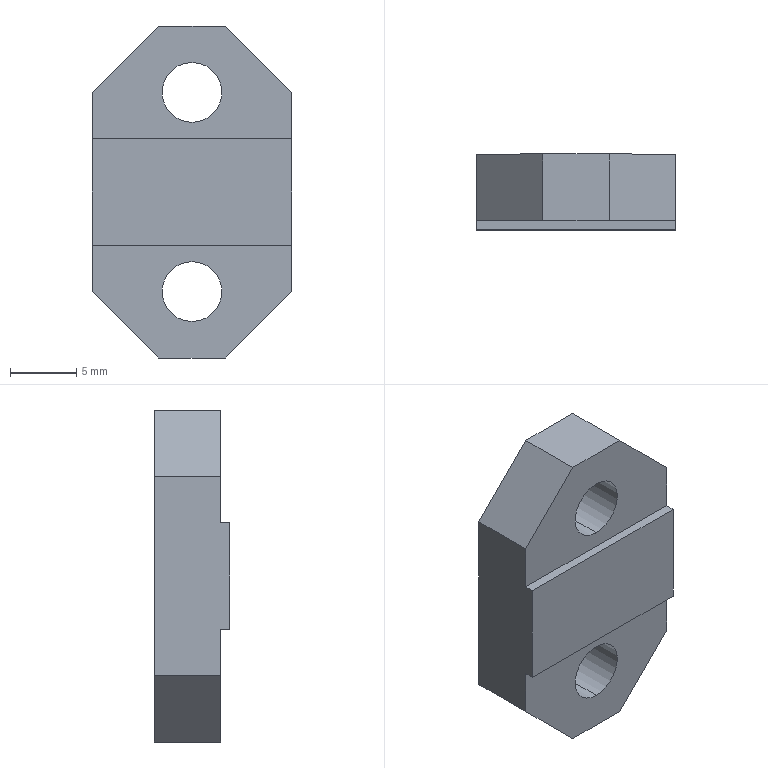Part | SolidWorks | features Chamfer 1, Extrusion 1, HoleWzd 1, ICE 1 | 1 solid | 18 faces | box 15 x 5.7 x 25 mm | volume 1550 mm3 | plane 14 | cylinder 4 | commonest cylinder face diameters 4.5 x4
STEP:
#1=CARTESIAN_POINT('',(0.,0.7,-9.75));
#2=VERTEX_POINT('',#1);
#3=CARTESIAN_POINT('',(0.,0.7,-5.25));
#4=VERTEX_POINT('',#3);
#5=CARTESIAN_POINT('',(0.,0.7,-7.5));
#6=DIRECTION('',(0.,1.,0.));
#7=DIRECTION('',(0.,0.,1.));
#8=AXIS2_PLACEMENT_3D('',#5,#6,#7);
#9=CIRCLE('',#8,2.25);
#10=EDGE_CURVE('',#2,#4,#9,.T.);
#11=ORIENTED_EDGE('',*,*,#10,.F.);
#12=CARTESIAN_POINT('',(0.,5.7,-9.75));
#13=VERTEX_POINT('',#12);
#14=CARTESIAN_POINT('',(0.,5.7,-9.75));
#15=DIRECTION('',(0.,1.,0.));
#16=VECTOR('',#15,1000.);
#17=LINE('',#14,#16);
#18=EDGE_CURVE('',#2,#13,#17,.T.);
#19=ORIENTED_EDGE('',*,*,#18,.T.);
#20=CARTESIAN_POINT('',(0.,5.7,-5.25));
#21=VERTEX_POINT('',#20);
#22=CARTESIAN_POINT('',(0.,5.7,-7.5));
#23=DIRECTION('',(0.,1.,0.));
#24=DIRECTION('',(0.,0.,1.));
#25=AXIS2_PLACEMENT_3D('',#22,#23,#24);
#26=CIRCLE('',#25,2.25);
#27=EDGE_CURVE('',#13,#21,#26,.T.);
#28=ORIENTED_EDGE('',*,*,#27,.T.);
#29=CARTESIAN_POINT('',(0.,5.7,-5.25));
#30=DIRECTION('',(0.,1.,0.));
#31=VECTOR('',#30,1000.);
#32=LINE('',#29,#31);
#33=EDGE_CURVE('',#4,#21,#32,.T.);
#34=ORIENTED_EDGE('',*,*,#33,.F.);
#35=EDGE_LOOP('',(#11,#19,#28,#34));
#36=FACE_OUTER_BOUND('',#35,.T.);
#37=CARTESIAN_POINT('',(0.,5.7,-7.5));
#38=DIRECTION('',(0.,1.,0.));
#39=DIRECTION('',(0.,0.,1.));
#40=AXIS2_PLACEMENT_3D('',#37,#38,#39);
#41=CYLINDRICAL_SURFACE('',#40,2.25);
#42=ADVANCED_FACE('',(#36),#41,.F.);
#43=CARTESIAN_POINT('',(0.,0.7,9.75));
#44=VERTEX_POINT('',#43);
#45=CARTESIAN_POINT('',(0.,0.7,5.25));
#46=VERTEX_POINT('',#45);
#47=CARTESIAN_POINT('',(0.,0.7,7.5));
#48=DIRECTION('',(0.,-1.,0.));
#49=DIRECTION('',(0.,0.,-1.));
#50=AXIS2_PLACEMENT_3D('',#47,#48,#49);
#51=CIRCLE('',#50,2.25);
#52=EDGE_CURVE('',#44,#46,#51,.T.);
#53=ORIENTED_EDGE('',*,*,#52,.T.);
#54=CARTESIAN_POINT('',(0.,5.7,5.25));
#55=VERTEX_POINT('',#54);
#56=CARTESIAN_POINT('',(0.,5.7,5.25));
#57=DIRECTION('',(0.,1.,0.));
#58=VECTOR('',#57,1000.);
#59=LINE('',#56,#58);
#60=EDGE_CURVE('',#46,#55,#59,.T.);
#61=ORIENTED_EDGE('',*,*,#60,.T.);
#62=CARTESIAN_POINT('',(0.,5.7,9.75));
#63=VERTEX_POINT('',#62);
#64=CARTESIAN_POINT('',(0.,5.7,7.5));
#65=DIRECTION('',(0.,1.,0.));
#66=DIRECTION('',(0.,0.,1.));
#67=AXIS2_PLACEMENT_3D('',#64,#65,#66);
#68=CIRCLE('',#67,2.25);
#69=EDGE_CURVE('',#55,#63,#68,.T.);
#70=ORIENTED_EDGE('',*,*,#69,.T.);
#71=CARTESIAN_POINT('',(0.,5.7,9.75));
#72=DIRECTION('',(0.,1.,0.));
#73=VECTOR('',#72,1000.);
#74=LINE('',#71,#73);
#75=EDGE_CURVE('',#44,#63,#74,.T.);
#76=ORIENTED_EDGE('',*,*,#75,.F.);
#77=EDGE_LOOP('',(#53,#61,#70,#76));
#78=FACE_OUTER_BOUND('',#77,.T.);
#79=CARTESIAN_POINT('',(0.,5.7,7.5));
#80=DIRECTION('',(0.,1.,0.));
#81=DIRECTION('',(0.,0.,1.));
#82=AXIS2_PLACEMENT_3D('',#79,#80,#81);
#83=CYLINDRICAL_SURFACE('',#82,2.25);
#84=ADVANCED_FACE('',(#78),#83,.F.);
#85=CARTESIAN_POINT('',(2.5,0.7,12.5));
#86=VERTEX_POINT('',#85);
#87=CARTESIAN_POINT('',(-2.5,0.7,12.5));
#88=VERTEX_POINT('',#87);
#89=CARTESIAN_POINT('',(-7.5,0.7,12.5));
#90=DIRECTION('',(-1.,0.,0.));
#91=VECTOR('',#90,1000.);
#92=LINE('',#89,#91);
#93=EDGE_CURVE('',#86,#88,#92,.T.);
#94=ORIENTED_EDGE('',*,*,#93,.F.);
#95=CARTESIAN_POINT('',(2.5,5.7,12.5));
#96=VERTEX_POINT('',#95);
#97=CARTESIAN_POINT('',(2.5,5.7,12.5));
#98=DIRECTION('',(0.,1.,0.));
#99=VECTOR('',#98,1000.);
#100=LINE('',#97,#99);
#101=EDGE_CURVE('',#86,#96,#100,.T.);
#102=ORIENTED_EDGE('',*,*,#101,.T.);
#103=CARTESIAN_POINT('',(-2.5,5.7,12.5));
#104=VERTEX_POINT('',#103);
#105=CARTESIAN_POINT('',(-7.5,5.7,12.5));
#106=DIRECTION('',(1.,0.,0.));
#107=VECTOR('',#106,1000.);
#108=LINE('',#105,#107);
#109=EDGE_CURVE('',#104,#96,#108,.T.);
#110=ORIENTED_EDGE('',*,*,#109,.F.);
#111=CARTESIAN_POINT('',(-2.5,5.7,12.5));
#112=DIRECTION('',(0.,-1.,0.));
#113=VECTOR('',#112,1000.);
#114=LINE('',#111,#113);
#115=EDGE_CURVE('',#104,#88,#114,.T.);
#116=ORIENTED_EDGE('',*,*,#115,.T.);
#117=EDGE_LOOP('',(#94,#102,#110,#116));
#118=FACE_OUTER_BOUND('',#117,.T.);
#119=CARTESIAN_POINT('',(-7.5,5.7,12.5));
#120=DIRECTION('',(0.,0.,-1.));
#121=DIRECTION('',(-1.,0.,0.));
#122=AXIS2_PLACEMENT_3D('',#119,#120,#121);
#123=PLANE('',#122);
#124=ADVANCED_FACE('',(#118),#123,.F.);
#125=CARTESIAN_POINT('',(7.5,5.7,7.5));
#126=VERTEX_POINT('',#125);
#127=CARTESIAN_POINT('',(7.5,5.7,-7.5));
#128=VERTEX_POINT('',#127);
#129=CARTESIAN_POINT('',(7.5,5.7,12.5));
#130=DIRECTION('',(0.,0.,-1.));
#131=VECTOR('',#130,1000.);
#132=LINE('',#129,#131);
#133=EDGE_CURVE('',#126,#128,#132,.T.);
#134=ORIENTED_EDGE('',*,*,#133,.F.);
#135=CARTESIAN_POINT('',(7.5,0.7,7.5));
#136=VERTEX_POINT('',#135);
#137=CARTESIAN_POINT('',(7.5,5.7,7.5));
#138=DIRECTION('',(0.,-1.,0.));
#139=VECTOR('',#138,1000.);
#140=LINE('',#137,#139);
#141=EDGE_CURVE('',#126,#136,#140,.T.);
#142=ORIENTED_EDGE('',*,*,#141,.T.);
#143=CARTESIAN_POINT('',(7.5,0.7,4.));
#144=VERTEX_POINT('',#143);
#145=CARTESIAN_POINT('',(7.5,0.7,12.5));
#146=DIRECTION('',(0.,0.,1.));
#147=VECTOR('',#146,1000.);
#148=LINE('',#145,#147);
#149=EDGE_CURVE('',#144,#136,#148,.T.);
#150=ORIENTED_EDGE('',*,*,#149,.F.);
#151=CARTESIAN_POINT('',(7.5,0.,4.));
#152=VERTEX_POINT('',#151);
#153=CARTESIAN_POINT('',(7.5,0.7,4.));
#154=DIRECTION('',(0.,-1.,0.));
#155=VECTOR('',#154,1000.);
#156=LINE('',#153,#155);
#157=EDGE_CURVE('',#144,#152,#156,.T.);
#158=ORIENTED_EDGE('',*,*,#157,.T.);
#159=CARTESIAN_POINT('',(7.5,0.,-4.));
#160=VERTEX_POINT('',#159);
#161=CARTESIAN_POINT('',(7.5,0.,12.5));
#162=DIRECTION('',(0.,0.,-1.));
#163=VECTOR('',#162,1000.);
#164=LINE('',#161,#163);
#165=EDGE_CURVE('',#152,#160,#164,.T.);
#166=ORIENTED_EDGE('',*,*,#165,.T.);
#167=CARTESIAN_POINT('',(7.5,0.7,-4.));
#168=VERTEX_POINT('',#167);
#169=CARTESIAN_POINT('',(7.5,0.7,-4.));
#170=DIRECTION('',(0.,-1.,0.));
#171=VECTOR('',#170,1000.);
#172=LINE('',#169,#171);
#173=EDGE_CURVE('',#168,#160,#172,.T.);
#174=ORIENTED_EDGE('',*,*,#173,.F.);
#175=CARTESIAN_POINT('',(7.5,0.7,-7.5));
#176=VERTEX_POINT('',#175);
#177=CARTESIAN_POINT('',(7.5,0.7,-12.5));
#178=DIRECTION('',(0.,0.,1.));
#179=VECTOR('',#178,1000.);
#180=LINE('',#177,#179);
#181=EDGE_CURVE('',#176,#168,#180,.T.);
#182=ORIENTED_EDGE('',*,*,#181,.F.);
#183=CARTESIAN_POINT('',(7.5,5.7,-7.5));
#184=DIRECTION('',(0.,1.,0.));
#185=VECTOR('',#184,1000.);
#186=LINE('',#183,#185);
#187=EDGE_CURVE('',#176,#128,#186,.T.);
#188=ORIENTED_EDGE('',*,*,#187,.T.);
#189=EDGE_LOOP('',(#134,#142,#150,#158,#166,#174,#182,#188));
#190=FACE_OUTER_BOUND('',#189,.T.);
#191=CARTESIAN_POINT('',(7.5,5.7,12.5));
#192=DIRECTION('',(-1.,0.,0.));
#193=DIRECTION('',(0.,0.,1.));
#194=AXIS2_PLACEMENT_3D('',#191,#192,#193);
#195=PLANE('',#194);
#196=ADVANCED_FACE('',(#190),#195,.F.);
#197=CARTESIAN_POINT('',(2.5,5.7,-12.5));
#198=VERTEX_POINT('',#197);
#199=CARTESIAN_POINT('',(-2.5,5.7,-12.5));
#200=VERTEX_POINT('',#199);
#201=CARTESIAN_POINT('',(-7.5,5.7,-12.5));
#202=DIRECTION('',(-1.,0.,0.));
#203=VECTOR('',#202,1000.);
#204=LINE('',#201,#203);
#205=EDGE_CURVE('',#198,#200,#204,.T.);
#206=ORIENTED_EDGE('',*,*,#205,.F.);
#207=CARTESIAN_POINT('',(2.5,0.7,-12.5));
#208=VERTEX_POINT('',#207);
#209=CARTESIAN_POINT('',(2.5,5.7,-12.5));
#210=DIRECTION('',(0.,-1.,0.));
#211=VECTOR('',#210,1000.);
#212=LINE('',#209,#211);
#213=EDGE_CURVE('',#198,#208,#212,.T.);
#214=ORIENTED_EDGE('',*,*,#213,.T.);
#215=CARTESIAN_POINT('',(-2.5,0.7,-12.5));
#216=VERTEX_POINT('',#215);
#217=CARTESIAN_POINT('',(-7.5,0.7,-12.5));
#218=DIRECTION('',(1.,0.,0.));
#219=VECTOR('',#218,1000.);
#220=LINE('',#217,#219);
#221=EDGE_CURVE('',#216,#208,#220,.T.);
#222=ORIENTED_EDGE('',*,*,#221,.F.);
#223=CARTESIAN_POINT('',(-2.5,5.7,-12.5));
#224=DIRECTION('',(0.,1.,0.));
#225=VECTOR('',#224,1000.);
#226=LINE('',#223,#225);
#227=EDGE_CURVE('',#216,#200,#226,.T.);
#228=ORIENTED_EDGE('',*,*,#227,.T.);
#229=EDGE_LOOP('',(#206,#214,#222,#228));
#230=FACE_OUTER_BOUND('',#229,.T.);
#231=CARTESIAN_POINT('',(-7.5,5.7,-12.5));
#232=DIRECTION('',(0.,0.,1.));
#233=DIRECTION('',(1.,0.,0.));
#234=AXIS2_PLACEMENT_3D('',#231,#232,#233);
#235=PLANE('',#234);
#236=ADVANCED_FACE('',(#230),#235,.F.);
#237=CARTESIAN_POINT('',(-7.5,0.7,7.5));
#238=VERTEX_POINT('',#237);
#239=CARTESIAN_POINT('',(-7.5,0.7,4.));
#240=VERTEX_POINT('',#239);
#241=CARTESIAN_POINT('',(-7.5,0.7,12.5));
#242=DIRECTION('',(0.,0.,-1.));
#243=VECTOR('',#242,1000.);
#244=LINE('',#241,#243);
#245=EDGE_CURVE('',#238,#240,#244,.T.);
#246=ORIENTED_EDGE('',*,*,#245,.F.);
#247=CARTESIAN_POINT('',(-7.5,5.7,7.5));
#248=VERTEX_POINT('',#247);
#249=CARTESIAN_POINT('',(-7.5,5.7,7.5));
#250=DIRECTION('',(0.,1.,0.));
#251=VECTOR('',#250,1000.);
#252=LINE('',#249,#251);
#253=EDGE_CURVE('',#238,#248,#252,.T.);
#254=ORIENTED_EDGE('',*,*,#253,.T.);
#255=CARTESIAN_POINT('',(-7.5,5.7,-7.5));
#256=VERTEX_POINT('',#255);
#257=CARTESIAN_POINT('',(-7.5,5.7,12.5));
#258=DIRECTION('',(0.,0.,1.));
#259=VECTOR('',#258,1000.);
#260=LINE('',#257,#259);
#261=EDGE_CURVE('',#256,#248,#260,.T.);
#262=ORIENTED_EDGE('',*,*,#261,.F.);
#263=CARTESIAN_POINT('',(-7.5,0.7,-7.5));
#264=VERTEX_POINT('',#263);
#265=CARTESIAN_POINT('',(-7.5,5.7,-7.5));
#266=DIRECTION('',(0.,-1.,0.));
#267=VECTOR('',#266,1000.);
#268=LINE('',#265,#267);
#269=EDGE_CURVE('',#256,#264,#268,.T.);
#270=ORIENTED_EDGE('',*,*,#269,.T.);
#271=CARTESIAN_POINT('',(-7.5,0.7,-4.));
#272=VERTEX_POINT('',#271);
#273=CARTESIAN_POINT('',(-7.5,0.7,-12.5));
#274=DIRECTION('',(0.,0.,-1.));
#275=VECTOR('',#274,1000.);
#276=LINE('',#273,#275);
#277=EDGE_CURVE('',#272,#264,#276,.T.);
#278=ORIENTED_EDGE('',*,*,#277,.F.);
#279=CARTESIAN_POINT('',(-7.5,0.,-4.));
#280=VERTEX_POINT('',#279);
#281=CARTESIAN_POINT('',(-7.5,0.7,-4.));
#282=DIRECTION('',(0.,-1.,0.));
#283=VECTOR('',#282,1000.);
#284=LINE('',#281,#283);
#285=EDGE_CURVE('',#272,#280,#284,.T.);
#286=ORIENTED_EDGE('',*,*,#285,.T.);
#287=CARTESIAN_POINT('',(-7.5,0.,4.));
#288=VERTEX_POINT('',#287);
#289=CARTESIAN_POINT('',(-7.5,0.,12.5));
#290=DIRECTION('',(0.,0.,1.));
#291=VECTOR('',#290,1000.);
#292=LINE('',#289,#291);
#293=EDGE_CURVE('',#280,#288,#292,.T.);
#294=ORIENTED_EDGE('',*,*,#293,.T.);
#295=CARTESIAN_POINT('',(-7.5,0.7,4.));
#296=DIRECTION('',(0.,-1.,0.));
#297=VECTOR('',#296,1000.);
#298=LINE('',#295,#297);
#299=EDGE_CURVE('',#240,#288,#298,.T.);
#300=ORIENTED_EDGE('',*,*,#299,.F.);
#301=EDGE_LOOP('',(#246,#254,#262,#270,#278,#286,#294,#300));
#302=FACE_OUTER_BOUND('',#301,.T.);
#303=CARTESIAN_POINT('',(-7.5,5.7,12.5));
#304=DIRECTION('',(1.,0.,0.));
#305=DIRECTION('',(0.,0.,-1.));
#306=AXIS2_PLACEMENT_3D('',#303,#304,#305);
#307=PLANE('',#306);
#308=ADVANCED_FACE('',(#302),#307,.F.);
#309=CARTESIAN_POINT('',(0.,5.7,-7.5));
#310=DIRECTION('',(0.,1.,0.));
#311=DIRECTION('',(0.,0.,1.));
#312=AXIS2_PLACEMENT_3D('',#309,#310,#311);
#313=CIRCLE('',#312,2.25);
#314=EDGE_CURVE('',#21,#13,#313,.T.);
#315=ORIENTED_EDGE('',*,*,#314,.F.);
#316=ORIENTED_EDGE('',*,*,#27,.F.);
#317=EDGE_LOOP('',(#315,#316));
#318=FACE_BOUND('',#317,.T.);
#319=CARTESIAN_POINT('',(0.,5.7,7.5));
#320=DIRECTION('',(0.,1.,0.));
#321=DIRECTION('',(0.,0.,1.));
#322=AXIS2_PLACEMENT_3D('',#319,#320,#321);
#323=CIRCLE('',#322,2.25);
#324=EDGE_CURVE('',#63,#55,#323,.T.);
#325=ORIENTED_EDGE('',*,*,#324,.F.);
#326=ORIENTED_EDGE('',*,*,#69,.F.);
#327=EDGE_LOOP('',(#325,#326));
#328=FACE_BOUND('',#327,.T.);
#329=ORIENTED_EDGE('',*,*,#109,.T.);
#330=CARTESIAN_POINT('',(7.5,5.7,7.5));
#331=DIRECTION('',(0.7071,0.,-0.7071));
#332=VECTOR('',#331,1000.);
#333=LINE('',#330,#332);
#334=EDGE_CURVE('',#96,#126,#333,.T.);
#335=ORIENTED_EDGE('',*,*,#334,.T.);
#336=ORIENTED_EDGE('',*,*,#133,.T.);
#337=CARTESIAN_POINT('',(2.5,5.7,-12.5));
#338=DIRECTION('',(-0.7071,0.,-0.7071));
#339=VECTOR('',#338,1000.);
#340=LINE('',#337,#339);
#341=EDGE_CURVE('',#128,#198,#340,.T.);
#342=ORIENTED_EDGE('',*,*,#341,.T.);
#343=ORIENTED_EDGE('',*,*,#205,.T.);
#344=CARTESIAN_POINT('',(-7.5,5.7,-7.5));
#345=DIRECTION('',(-0.7071,0.,0.7071));
#346=VECTOR('',#345,1000.);
#347=LINE('',#344,#346);
#348=EDGE_CURVE('',#200,#256,#347,.T.);
#349=ORIENTED_EDGE('',*,*,#348,.T.);
#350=ORIENTED_EDGE('',*,*,#261,.T.);
#351=CARTESIAN_POINT('',(-2.5,5.7,12.5));
#352=DIRECTION('',(0.7071,0.,0.7071));
#353=VECTOR('',#352,1000.);
#354=LINE('',#351,#353);
#355=EDGE_CURVE('',#248,#104,#354,.T.);
#356=ORIENTED_EDGE('',*,*,#355,.T.);
#357=EDGE_LOOP('',(#329,#335,#336,#342,#343,#349,#350,#356));
#358=FACE_OUTER_BOUND('',#357,.T.);
#359=CARTESIAN_POINT('',(0.,5.7,0.));
#360=DIRECTION('',(0.,-1.,0.));
#361=DIRECTION('',(0.,0.,-1.));
#362=AXIS2_PLACEMENT_3D('',#359,#360,#361);
#363=PLANE('',#362);
#364=ADVANCED_FACE('',(#318,#328,#358),#363,.F.);
#365=CARTESIAN_POINT('',(-7.5,0.,-4.));
#366=DIRECTION('',(-1.,0.,0.));
#367=VECTOR('',#366,1000.);
#368=LINE('',#365,#367);
#369=EDGE_CURVE('',#160,#280,#368,.T.);
#370=ORIENTED_EDGE('',*,*,#369,.F.);
#371=ORIENTED_EDGE('',*,*,#165,.F.);
#372=CARTESIAN_POINT('',(-7.5,0.,4.));
#373=DIRECTION('',(1.,0.,0.));
#374=VECTOR('',#373,1000.);
#375=LINE('',#372,#374);
#376=EDGE_CURVE('',#288,#152,#375,.T.);
#377=ORIENTED_EDGE('',*,*,#376,.F.);
#378=ORIENTED_EDGE('',*,*,#293,.F.);
#379=EDGE_LOOP('',(#370,#371,#377,#378));
#380=FACE_OUTER_BOUND('',#379,.T.);
#381=CARTESIAN_POINT('',(0.,0.,0.));
#382=DIRECTION('',(0.,-1.,0.));
#383=DIRECTION('',(0.,0.,-1.));
#384=AXIS2_PLACEMENT_3D('',#381,#382,#383);
#385=PLANE('',#384);
#386=ADVANCED_FACE('',(#380),#385,.T.);
#387=ORIENTED_EDGE('',*,*,#376,.T.);
#388=ORIENTED_EDGE('',*,*,#157,.F.);
#389=CARTESIAN_POINT('',(-7.5,0.7,4.));
#390=DIRECTION('',(1.,0.,0.));
#391=VECTOR('',#390,1000.);
#392=LINE('',#389,#391);
#393=EDGE_CURVE('',#240,#144,#392,.T.);
#394=ORIENTED_EDGE('',*,*,#393,.F.);
#395=ORIENTED_EDGE('',*,*,#299,.T.);
#396=EDGE_LOOP('',(#387,#388,#394,#395));
#397=FACE_OUTER_BOUND('',#396,.T.);
#398=CARTESIAN_POINT('',(-7.5,0.7,4.));
#399=DIRECTION('',(0.,0.,-1.));
#400=DIRECTION('',(-1.,0.,0.));
#401=AXIS2_PLACEMENT_3D('',#398,#399,#400);
#402=PLANE('',#401);
#403=ADVANCED_FACE('',(#397),#402,.F.);
#404=ORIENTED_EDGE('',*,*,#52,.F.);
#405=CARTESIAN_POINT('',(0.,0.7,7.5));
#406=DIRECTION('',(0.,-1.,0.));
#407=DIRECTION('',(0.,0.,-1.));
#408=AXIS2_PLACEMENT_3D('',#405,#406,#407);
#409=CIRCLE('',#408,2.25);
#410=EDGE_CURVE('',#46,#44,#409,.T.);
#411=ORIENTED_EDGE('',*,*,#410,.F.);
#412=EDGE_LOOP('',(#404,#411));
#413=FACE_BOUND('',#412,.T.);
#414=ORIENTED_EDGE('',*,*,#149,.T.);
#415=CARTESIAN_POINT('',(7.5,0.7,7.5));
#416=DIRECTION('',(-0.7071,0.,0.7071));
#417=VECTOR('',#416,1000.);
#418=LINE('',#415,#417);
#419=EDGE_CURVE('',#136,#86,#418,.T.);
#420=ORIENTED_EDGE('',*,*,#419,.T.);
#421=ORIENTED_EDGE('',*,*,#93,.T.);
#422=CARTESIAN_POINT('',(-7.5,0.7,7.5));
#423=DIRECTION('',(-0.7071,0.,-0.7071));
#424=VECTOR('',#423,1000.);
#425=LINE('',#422,#424);
#426=EDGE_CURVE('',#88,#238,#425,.T.);
#427=ORIENTED_EDGE('',*,*,#426,.T.);
#428=ORIENTED_EDGE('',*,*,#245,.T.);
#429=ORIENTED_EDGE('',*,*,#393,.T.);
#430=EDGE_LOOP('',(#414,#420,#421,#427,#428,#429));
#431=FACE_OUTER_BOUND('',#430,.T.);
#432=CARTESIAN_POINT('',(0.,0.7,0.));
#433=DIRECTION('',(0.,-1.,0.));
#434=DIRECTION('',(0.,0.,-1.));
#435=AXIS2_PLACEMENT_3D('',#432,#433,#434);
#436=PLANE('',#435);
#437=ADVANCED_FACE('',(#413,#431),#436,.T.);
#438=ORIENTED_EDGE('',*,*,#369,.T.);
#439=ORIENTED_EDGE('',*,*,#285,.F.);
#440=CARTESIAN_POINT('',(-7.5,0.7,-4.));
#441=DIRECTION('',(-1.,0.,0.));
#442=VECTOR('',#441,1000.);
#443=LINE('',#440,#442);
#444=EDGE_CURVE('',#168,#272,#443,.T.);
#445=ORIENTED_EDGE('',*,*,#444,.F.);
#446=ORIENTED_EDGE('',*,*,#173,.T.);
#447=EDGE_LOOP('',(#438,#439,#445,#446));
#448=FACE_OUTER_BOUND('',#447,.T.);
#449=CARTESIAN_POINT('',(-7.5,0.7,-4.));
#450=DIRECTION('',(0.,0.,1.));
#451=DIRECTION('',(1.,0.,0.));
#452=AXIS2_PLACEMENT_3D('',#449,#450,#451);
#453=PLANE('',#452);
#454=ADVANCED_FACE('',(#448),#453,.F.);
#455=CARTESIAN_POINT('',(0.,0.7,-7.5));
#456=DIRECTION('',(0.,1.,0.));
#457=DIRECTION('',(0.,0.,1.));
#458=AXIS2_PLACEMENT_3D('',#455,#456,#457);
#459=CIRCLE('',#458,2.25);
#460=EDGE_CURVE('',#4,#2,#459,.T.);
#461=ORIENTED_EDGE('',*,*,#460,.T.);
#462=ORIENTED_EDGE('',*,*,#10,.T.);
#463=EDGE_LOOP('',(#461,#462));
#464=FACE_BOUND('',#463,.T.);
#465=ORIENTED_EDGE('',*,*,#221,.T.);
#466=CARTESIAN_POINT('',(2.5,0.7,-12.5));
#467=DIRECTION('',(0.7071,0.,0.7071));
#468=VECTOR('',#467,1000.);
#469=LINE('',#466,#468);
#470=EDGE_CURVE('',#208,#176,#469,.T.);
#471=ORIENTED_EDGE('',*,*,#470,.T.);
#472=ORIENTED_EDGE('',*,*,#181,.T.);
#473=ORIENTED_EDGE('',*,*,#444,.T.);
#474=ORIENTED_EDGE('',*,*,#277,.T.);
#475=CARTESIAN_POINT('',(-7.5,0.7,-7.5));
#476=DIRECTION('',(0.7071,0.,-0.7071));
#477=VECTOR('',#476,1000.);
#478=LINE('',#475,#477);
#479=EDGE_CURVE('',#264,#216,#478,.T.);
#480=ORIENTED_EDGE('',*,*,#479,.T.);
#481=EDGE_LOOP('',(#465,#471,#472,#473,#474,#480));
#482=FACE_OUTER_BOUND('',#481,.T.);
#483=CARTESIAN_POINT('',(0.,0.7,0.));
#484=DIRECTION('',(0.,1.,0.));
#485=DIRECTION('',(0.,0.,1.));
#486=AXIS2_PLACEMENT_3D('',#483,#484,#485);
#487=PLANE('',#486);
#488=ADVANCED_FACE('',(#464,#482),#487,.F.);
#489=ORIENTED_EDGE('',*,*,#334,.F.);
#490=ORIENTED_EDGE('',*,*,#101,.F.);
#491=ORIENTED_EDGE('',*,*,#419,.F.);
#492=ORIENTED_EDGE('',*,*,#141,.F.);
#493=EDGE_LOOP('',(#489,#490,#491,#492));
#494=FACE_OUTER_BOUND('',#493,.T.);
#495=CARTESIAN_POINT('',(7.5,5.7,7.5));
#496=DIRECTION('',(-0.7071,0.,-0.7071));
#497=DIRECTION('',(0.,-1.,0.));
#498=AXIS2_PLACEMENT_3D('',#495,#496,#497);
#499=PLANE('',#498);
#500=ADVANCED_FACE('',(#494),#499,.F.);
#501=ORIENTED_EDGE('',*,*,#355,.F.);
#502=ORIENTED_EDGE('',*,*,#253,.F.);
#503=ORIENTED_EDGE('',*,*,#426,.F.);
#504=ORIENTED_EDGE('',*,*,#115,.F.);
#505=EDGE_LOOP('',(#501,#502,#503,#504));
#506=FACE_OUTER_BOUND('',#505,.T.);
#507=CARTESIAN_POINT('',(-2.5,5.7,12.5));
#508=DIRECTION('',(0.7071,0.,-0.7071));
#509=DIRECTION('',(0.,-1.,0.));
#510=AXIS2_PLACEMENT_3D('',#507,#508,#509);
#511=PLANE('',#510);
#512=ADVANCED_FACE('',(#506),#511,.F.);
#513=ORIENTED_EDGE('',*,*,#341,.F.);
#514=ORIENTED_EDGE('',*,*,#187,.F.);
#515=ORIENTED_EDGE('',*,*,#470,.F.);
#516=ORIENTED_EDGE('',*,*,#213,.F.);
#517=EDGE_LOOP('',(#513,#514,#515,#516));
#518=FACE_OUTER_BOUND('',#517,.T.);
#519=CARTESIAN_POINT('',(2.5,5.7,-12.5));
#520=DIRECTION('',(-0.7071,0.,0.7071));
#521=DIRECTION('',(0.,-1.,0.));
#522=AXIS2_PLACEMENT_3D('',#519,#520,#521);
#523=PLANE('',#522);
#524=ADVANCED_FACE('',(#518),#523,.F.);
#525=ORIENTED_EDGE('',*,*,#348,.F.);
#526=ORIENTED_EDGE('',*,*,#227,.F.);
#527=ORIENTED_EDGE('',*,*,#479,.F.);
#528=ORIENTED_EDGE('',*,*,#269,.F.);
#529=EDGE_LOOP('',(#525,#526,#527,#528));
#530=FACE_OUTER_BOUND('',#529,.T.);
#531=CARTESIAN_POINT('',(-7.5,5.7,-7.5));
#532=DIRECTION('',(0.7071,0.,0.7071));
#533=DIRECTION('',(0.,-1.,0.));
#534=AXIS2_PLACEMENT_3D('',#531,#532,#533);
#535=PLANE('',#534);
#536=ADVANCED_FACE('',(#530),#535,.F.);
#537=ORIENTED_EDGE('',*,*,#60,.F.);
#538=ORIENTED_EDGE('',*,*,#410,.T.);
#539=ORIENTED_EDGE('',*,*,#75,.T.);
#540=ORIENTED_EDGE('',*,*,#324,.T.);
#541=EDGE_LOOP('',(#537,#538,#539,#540));
#542=FACE_OUTER_BOUND('',#541,.T.);
#543=CARTESIAN_POINT('',(0.,5.7,7.5));
#544=DIRECTION('',(0.,1.,0.));
#545=DIRECTION('',(0.,0.,1.));
#546=AXIS2_PLACEMENT_3D('',#543,#544,#545);
#547=CYLINDRICAL_SURFACE('',#546,2.25);
#548=ADVANCED_FACE('',(#542),#547,.F.);
#549=ORIENTED_EDGE('',*,*,#18,.F.);
#550=ORIENTED_EDGE('',*,*,#460,.F.);
#551=ORIENTED_EDGE('',*,*,#33,.T.);
#552=ORIENTED_EDGE('',*,*,#314,.T.);
#553=EDGE_LOOP('',(#549,#550,#551,#552));
#554=FACE_OUTER_BOUND('',#553,.T.);
#555=CARTESIAN_POINT('',(0.,5.7,-7.5));
#556=DIRECTION('',(0.,1.,0.));
#557=DIRECTION('',(0.,0.,1.));
#558=AXIS2_PLACEMENT_3D('',#555,#556,#557);
#559=CYLINDRICAL_SURFACE('',#558,2.25);
#560=ADVANCED_FACE('',(#554),#559,.F.);
#561=CLOSED_SHELL('',(#42,#84,#124,#196,#236,#308,#364,#386,#403,#437,#454,#488,#500,#512,#524,#536,#548,#560));
#562=MANIFOLD_SOLID_BREP('',#561);
#563=CARTESIAN_POINT('',(0.,0.,0.));
#564=DIRECTION('',(0.,0.,1.));
#565=DIRECTION('',(1.,0.,0.));
#566=AXIS2_PLACEMENT_3D('',#563,#564,#565);
#567=(LENGTH_UNIT()NAMED_UNIT(*)SI_UNIT(.MILLI.,.METRE.));
#568=UNCERTAINTY_MEASURE_WITH_UNIT(LENGTH_MEASURE(0.00001),#567,'','');
#569=(NAMED_UNIT(*)PLANE_ANGLE_UNIT()SI_UNIT($,.RADIAN.));
#570=(NAMED_UNIT(*)SI_UNIT($,.STERADIAN.)SOLID_ANGLE_UNIT());
#571=(GEOMETRIC_REPRESENTATION_CONTEXT(3)GLOBAL_UNCERTAINTY_ASSIGNED_CONTEXT((#568))GLOBAL_UNIT_ASSIGNED_CONTEXT((#567,#569,#570))REPRESENTATION_CONTEXT('',''));
#572=ADVANCED_BREP_SHAPE_REPRESENTATION('',(#562,#566),#571);